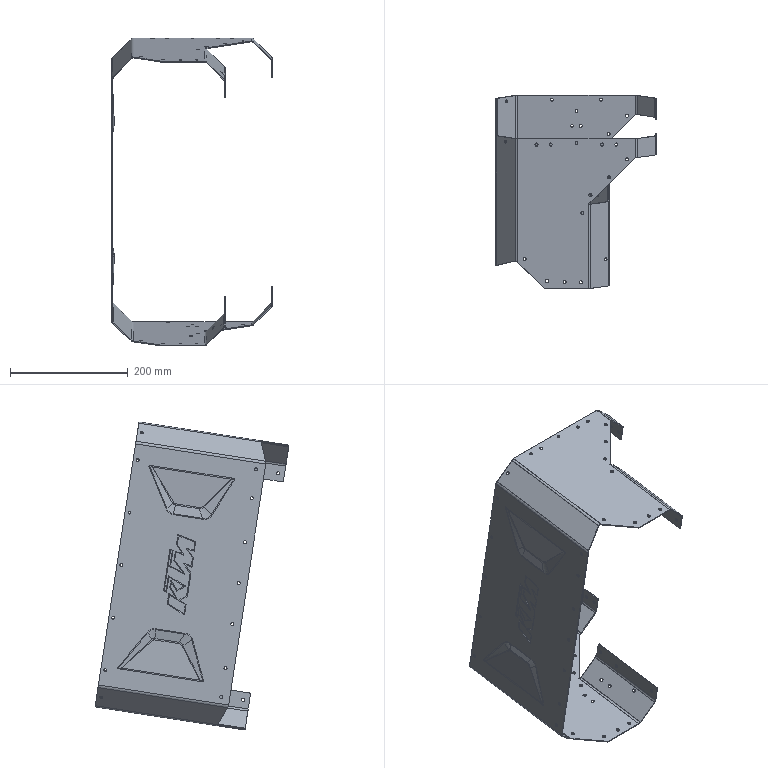Part | SolidWorks | features BaseBody 1 | 1 solid | 315 faces | box 273.497 x 329.581 x 523.596 mm | volume 319400 mm3 | cylinder 154 | plane 84 | spline 77 | commonest cylinder face diameters 5.2 x82 4.9 x30 13 x13 10 x12 4 x11 1.905 x3